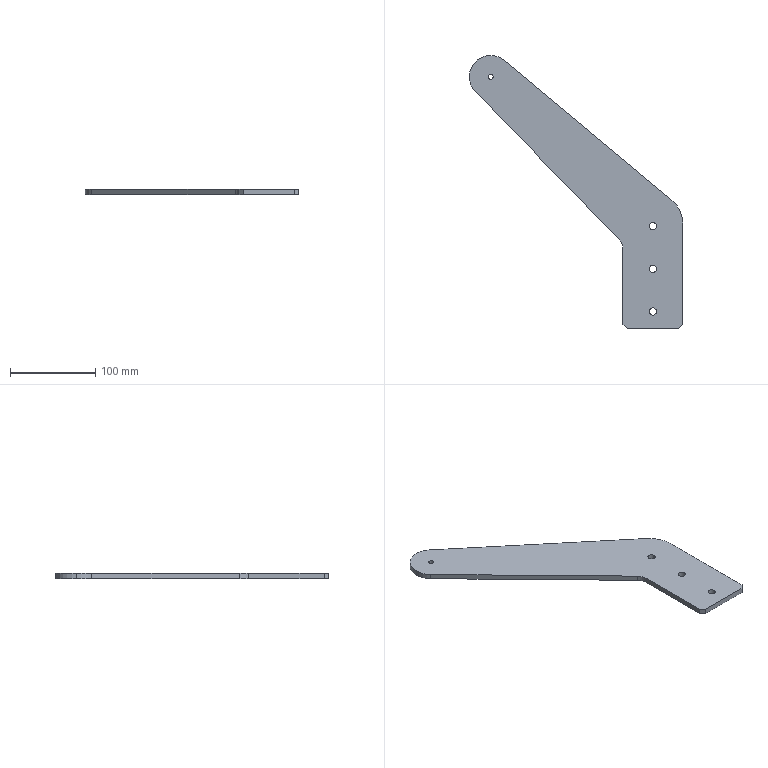Part | SolidWorks | features Chamfer 1, Extrusion 1 | 1 solid | 21 faces | box 250 x 320 x 6 mm | volume 153103 mm3 | cylinder 12 | plane 9 | commonest cylinder face diameters 8.5 x6 6 x2 50 x2 30 x1 70 x1
STEP:
#1=CARTESIAN_POINT('',(185.75,-175.,6.));
#2=VERTEX_POINT('',#1);
#3=CARTESIAN_POINT('',(194.25,-175.,6.));
#4=VERTEX_POINT('',#3);
#5=CARTESIAN_POINT('',(190.,-175.,6.));
#6=DIRECTION('',(0.,0.,1.));
#7=DIRECTION('',(1.,0.,0.));
#8=AXIS2_PLACEMENT_3D('',#5,#6,#7);
#9=CIRCLE('',#8,4.25);
#10=EDGE_CURVE('',#2,#4,#9,.T.);
#11=ORIENTED_EDGE('',*,*,#10,.T.);
#12=CARTESIAN_POINT('',(194.25,-175.,0.));
#13=VERTEX_POINT('',#12);
#14=CARTESIAN_POINT('',(194.25,-175.,6.));
#15=DIRECTION('',(0.,0.,-1.));
#16=VECTOR('',#15,1000.);
#17=LINE('',#14,#16);
#18=EDGE_CURVE('',#4,#13,#17,.T.);
#19=ORIENTED_EDGE('',*,*,#18,.T.);
#20=CARTESIAN_POINT('',(185.75,-175.,0.));
#21=VERTEX_POINT('',#20);
#22=CARTESIAN_POINT('',(190.,-175.,0.));
#23=DIRECTION('',(0.,0.,1.));
#24=DIRECTION('',(1.,0.,0.));
#25=AXIS2_PLACEMENT_3D('',#22,#23,#24);
#26=CIRCLE('',#25,4.25);
#27=EDGE_CURVE('',#21,#13,#26,.T.);
#28=ORIENTED_EDGE('',*,*,#27,.F.);
#29=CARTESIAN_POINT('',(185.75,-175.,6.));
#30=DIRECTION('',(0.,0.,-1.));
#31=VECTOR('',#30,1000.);
#32=LINE('',#29,#31);
#33=EDGE_CURVE('',#2,#21,#32,.T.);
#34=ORIENTED_EDGE('',*,*,#33,.F.);
#35=EDGE_LOOP('',(#11,#19,#28,#34));
#36=FACE_OUTER_BOUND('',#35,.T.);
#37=CARTESIAN_POINT('',(190.,-175.,6.));
#38=DIRECTION('',(0.,0.,-1.));
#39=DIRECTION('',(-1.,0.,0.));
#40=AXIS2_PLACEMENT_3D('',#37,#38,#39);
#41=CYLINDRICAL_SURFACE('',#40,4.25);
#42=ADVANCED_FACE('',(#36),#41,.F.);
#43=CARTESIAN_POINT('',(185.75,-225.,6.));
#44=VERTEX_POINT('',#43);
#45=CARTESIAN_POINT('',(194.25,-225.,6.));
#46=VERTEX_POINT('',#45);
#47=CARTESIAN_POINT('',(190.,-225.,6.));
#48=DIRECTION('',(0.,0.,1.));
#49=DIRECTION('',(1.,0.,0.));
#50=AXIS2_PLACEMENT_3D('',#47,#48,#49);
#51=CIRCLE('',#50,4.25);
#52=EDGE_CURVE('',#44,#46,#51,.T.);
#53=ORIENTED_EDGE('',*,*,#52,.T.);
#54=CARTESIAN_POINT('',(194.25,-225.,0.));
#55=VERTEX_POINT('',#54);
#56=CARTESIAN_POINT('',(194.25,-225.,6.));
#57=DIRECTION('',(0.,0.,-1.));
#58=VECTOR('',#57,1000.);
#59=LINE('',#56,#58);
#60=EDGE_CURVE('',#46,#55,#59,.T.);
#61=ORIENTED_EDGE('',*,*,#60,.T.);
#62=CARTESIAN_POINT('',(185.75,-225.,0.));
#63=VERTEX_POINT('',#62);
#64=CARTESIAN_POINT('',(190.,-225.,0.));
#65=DIRECTION('',(0.,0.,1.));
#66=DIRECTION('',(1.,0.,0.));
#67=AXIS2_PLACEMENT_3D('',#64,#65,#66);
#68=CIRCLE('',#67,4.25);
#69=EDGE_CURVE('',#63,#55,#68,.T.);
#70=ORIENTED_EDGE('',*,*,#69,.F.);
#71=CARTESIAN_POINT('',(185.75,-225.,6.));
#72=DIRECTION('',(0.,0.,-1.));
#73=VECTOR('',#72,1000.);
#74=LINE('',#71,#73);
#75=EDGE_CURVE('',#44,#63,#74,.T.);
#76=ORIENTED_EDGE('',*,*,#75,.F.);
#77=EDGE_LOOP('',(#53,#61,#70,#76));
#78=FACE_OUTER_BOUND('',#77,.T.);
#79=CARTESIAN_POINT('',(190.,-225.,6.));
#80=DIRECTION('',(0.,0.,-1.));
#81=DIRECTION('',(-1.,0.,0.));
#82=AXIS2_PLACEMENT_3D('',#79,#80,#81);
#83=CYLINDRICAL_SURFACE('',#82,4.25);
#84=ADVANCED_FACE('',(#78),#83,.F.);
#85=CARTESIAN_POINT('',(185.75,-275.,6.));
#86=VERTEX_POINT('',#85);
#87=CARTESIAN_POINT('',(194.25,-275.,6.));
#88=VERTEX_POINT('',#87);
#89=CARTESIAN_POINT('',(190.,-275.,6.));
#90=DIRECTION('',(0.,0.,1.));
#91=DIRECTION('',(1.,0.,0.));
#92=AXIS2_PLACEMENT_3D('',#89,#90,#91);
#93=CIRCLE('',#92,4.25);
#94=EDGE_CURVE('',#86,#88,#93,.T.);
#95=ORIENTED_EDGE('',*,*,#94,.T.);
#96=CARTESIAN_POINT('',(194.25,-275.,0.));
#97=VERTEX_POINT('',#96);
#98=CARTESIAN_POINT('',(194.25,-275.,6.));
#99=DIRECTION('',(0.,0.,-1.));
#100=VECTOR('',#99,1000.);
#101=LINE('',#98,#100);
#102=EDGE_CURVE('',#88,#97,#101,.T.);
#103=ORIENTED_EDGE('',*,*,#102,.T.);
#104=CARTESIAN_POINT('',(185.75,-275.,0.));
#105=VERTEX_POINT('',#104);
#106=CARTESIAN_POINT('',(190.,-275.,0.));
#107=DIRECTION('',(0.,0.,1.));
#108=DIRECTION('',(1.,0.,0.));
#109=AXIS2_PLACEMENT_3D('',#106,#107,#108);
#110=CIRCLE('',#109,4.25);
#111=EDGE_CURVE('',#105,#97,#110,.T.);
#112=ORIENTED_EDGE('',*,*,#111,.F.);
#113=CARTESIAN_POINT('',(185.75,-275.,6.));
#114=DIRECTION('',(0.,0.,-1.));
#115=VECTOR('',#114,1000.);
#116=LINE('',#113,#115);
#117=EDGE_CURVE('',#86,#105,#116,.T.);
#118=ORIENTED_EDGE('',*,*,#117,.F.);
#119=EDGE_LOOP('',(#95,#103,#112,#118));
#120=FACE_OUTER_BOUND('',#119,.T.);
#121=CARTESIAN_POINT('',(190.,-275.,6.));
#122=DIRECTION('',(0.,0.,-1.));
#123=DIRECTION('',(-1.,0.,0.));
#124=AXIS2_PLACEMENT_3D('',#121,#122,#123);
#125=CYLINDRICAL_SURFACE('',#124,4.25);
#126=ADVANCED_FACE('',(#120),#125,.F.);
#127=CARTESIAN_POINT('',(-3.,0.,6.));
#128=VERTEX_POINT('',#127);
#129=CARTESIAN_POINT('',(3.,0.,6.));
#130=VERTEX_POINT('',#129);
#131=CARTESIAN_POINT('',(0.,0.,6.));
#132=DIRECTION('',(0.,0.,1.));
#133=DIRECTION('',(1.,0.,0.));
#134=AXIS2_PLACEMENT_3D('',#131,#132,#133);
#135=CIRCLE('',#134,3.);
#136=EDGE_CURVE('',#128,#130,#135,.T.);
#137=ORIENTED_EDGE('',*,*,#136,.T.);
#138=CARTESIAN_POINT('',(3.,0.,0.));
#139=VERTEX_POINT('',#138);
#140=CARTESIAN_POINT('',(3.,0.,6.));
#141=DIRECTION('',(0.,0.,-1.));
#142=VECTOR('',#141,1000.);
#143=LINE('',#140,#142);
#144=EDGE_CURVE('',#130,#139,#143,.T.);
#145=ORIENTED_EDGE('',*,*,#144,.T.);
#146=CARTESIAN_POINT('',(-3.,0.,0.));
#147=VERTEX_POINT('',#146);
#148=CARTESIAN_POINT('',(0.,0.,0.));
#149=DIRECTION('',(0.,0.,1.));
#150=DIRECTION('',(1.,0.,0.));
#151=AXIS2_PLACEMENT_3D('',#148,#149,#150);
#152=CIRCLE('',#151,3.);
#153=EDGE_CURVE('',#147,#139,#152,.T.);
#154=ORIENTED_EDGE('',*,*,#153,.F.);
#155=CARTESIAN_POINT('',(-3.,0.,6.));
#156=DIRECTION('',(0.,0.,-1.));
#157=VECTOR('',#156,1000.);
#158=LINE('',#155,#157);
#159=EDGE_CURVE('',#128,#147,#158,.T.);
#160=ORIENTED_EDGE('',*,*,#159,.F.);
#161=EDGE_LOOP('',(#137,#145,#154,#160));
#162=FACE_OUTER_BOUND('',#161,.T.);
#163=CARTESIAN_POINT('',(0.,0.,6.));
#164=DIRECTION('',(0.,0.,-1.));
#165=DIRECTION('',(-1.,0.,0.));
#166=AXIS2_PLACEMENT_3D('',#163,#164,#165);
#167=CYLINDRICAL_SURFACE('',#166,3.);
#168=ADVANCED_FACE('',(#162),#167,.F.);
#169=CARTESIAN_POINT('',(-25.,0.,6.));
#170=VERTEX_POINT('',#169);
#171=CARTESIAN_POINT('',(-17.911,-17.442,6.));
#172=VERTEX_POINT('',#171);
#173=CARTESIAN_POINT('',(0.,0.,6.));
#174=DIRECTION('',(0.,0.,1.));
#175=DIRECTION('',(1.,0.,0.));
#176=AXIS2_PLACEMENT_3D('',#173,#174,#175);
#177=CIRCLE('',#176,25.);
#178=EDGE_CURVE('',#170,#172,#177,.T.);
#179=ORIENTED_EDGE('',*,*,#178,.F.);
#180=CARTESIAN_POINT('',(-25.,0.,0.));
#181=VERTEX_POINT('',#180);
#182=CARTESIAN_POINT('',(-25.,0.,6.));
#183=DIRECTION('',(0.,0.,-1.));
#184=VECTOR('',#183,1000.);
#185=LINE('',#182,#184);
#186=EDGE_CURVE('',#170,#181,#185,.T.);
#187=ORIENTED_EDGE('',*,*,#186,.T.);
#188=CARTESIAN_POINT('',(-17.911,-17.442,0.));
#189=VERTEX_POINT('',#188);
#190=CARTESIAN_POINT('',(0.,0.,0.));
#191=DIRECTION('',(0.,0.,1.));
#192=DIRECTION('',(1.,0.,0.));
#193=AXIS2_PLACEMENT_3D('',#190,#191,#192);
#194=CIRCLE('',#193,25.);
#195=EDGE_CURVE('',#181,#189,#194,.T.);
#196=ORIENTED_EDGE('',*,*,#195,.T.);
#197=CARTESIAN_POINT('',(-17.911,-17.442,6.));
#198=DIRECTION('',(0.,0.,-1.));
#199=VECTOR('',#198,1000.);
#200=LINE('',#197,#199);
#201=EDGE_CURVE('',#172,#189,#200,.T.);
#202=ORIENTED_EDGE('',*,*,#201,.F.);
#203=EDGE_LOOP('',(#179,#187,#196,#202));
#204=FACE_OUTER_BOUND('',#203,.T.);
#205=CARTESIAN_POINT('',(0.,0.,6.));
#206=DIRECTION('',(0.,0.,-1.));
#207=DIRECTION('',(-1.,0.,0.));
#208=AXIS2_PLACEMENT_3D('',#205,#206,#207);
#209=CYLINDRICAL_SURFACE('',#208,25.);
#210=ADVANCED_FACE('',(#204),#209,.T.);
#211=ORIENTED_EDGE('',*,*,#52,.F.);
#212=CARTESIAN_POINT('',(190.,-225.,6.));
#213=DIRECTION('',(0.,0.,1.));
#214=DIRECTION('',(1.,0.,0.));
#215=AXIS2_PLACEMENT_3D('',#212,#213,#214);
#216=CIRCLE('',#215,4.25);
#217=EDGE_CURVE('',#46,#44,#216,.T.);
#218=ORIENTED_EDGE('',*,*,#217,.F.);
#219=EDGE_LOOP('',(#211,#218));
#220=FACE_BOUND('',#219,.T.);
#221=ORIENTED_EDGE('',*,*,#136,.F.);
#222=CARTESIAN_POINT('',(0.,0.,6.));
#223=DIRECTION('',(0.,0.,1.));
#224=DIRECTION('',(1.,0.,0.));
#225=AXIS2_PLACEMENT_3D('',#222,#223,#224);
#226=CIRCLE('',#225,3.);
#227=EDGE_CURVE('',#130,#128,#226,.T.);
#228=ORIENTED_EDGE('',*,*,#227,.F.);
#229=EDGE_LOOP('',(#221,#228));
#230=FACE_BOUND('',#229,.T.);
#231=CARTESIAN_POINT('',(160.,-295.,6.));
#232=VERTEX_POINT('',#231);
#233=CARTESIAN_POINT('',(220.,-295.,6.));
#234=VERTEX_POINT('',#233);
#235=CARTESIAN_POINT('',(225.,-295.,6.));
#236=DIRECTION('',(1.,0.,0.));
#237=VECTOR('',#236,1000.);
#238=LINE('',#235,#237);
#239=EDGE_CURVE('',#232,#234,#238,.T.);
#240=ORIENTED_EDGE('',*,*,#239,.T.);
#241=CARTESIAN_POINT('',(225.,-290.,6.));
#242=VERTEX_POINT('',#241);
#243=CARTESIAN_POINT('',(257.5,-257.5,6.));
#244=DIRECTION('',(0.7071,0.7071,0.));
#245=VECTOR('',#244,1000.);
#246=LINE('',#243,#245);
#247=EDGE_CURVE('',#234,#242,#246,.T.);
#248=ORIENTED_EDGE('',*,*,#247,.T.);
#249=CARTESIAN_POINT('',(225.,-171.391,6.));
#250=VERTEX_POINT('',#249);
#251=CARTESIAN_POINT('',(225.,-171.391,6.));
#252=DIRECTION('',(0.,1.,0.));
#253=VECTOR('',#252,1000.);
#254=LINE('',#251,#253);
#255=EDGE_CURVE('',#242,#250,#254,.T.);
#256=ORIENTED_EDGE('',*,*,#255,.T.);
#257=CARTESIAN_POINT('',(212.41,-144.506,6.));
#258=VERTEX_POINT('',#257);
#259=CARTESIAN_POINT('',(190.,-171.391,6.));
#260=DIRECTION('',(0.,0.,1.));
#261=DIRECTION('',(-1.,0.,0.));
#262=AXIS2_PLACEMENT_3D('',#259,#260,#261);
#263=CIRCLE('',#262,35.);
#264=EDGE_CURVE('',#250,#258,#263,.T.);
#265=ORIENTED_EDGE('',*,*,#264,.T.);
#266=CARTESIAN_POINT('',(16.007,19.204,6.));
#267=VERTEX_POINT('',#266);
#268=CARTESIAN_POINT('',(16.007,19.204,6.));
#269=DIRECTION('',(-0.7681,0.6403,0.));
#270=VECTOR('',#269,1000.);
#271=LINE('',#268,#270);
#272=EDGE_CURVE('',#258,#267,#271,.T.);
#273=ORIENTED_EDGE('',*,*,#272,.T.);
#274=CARTESIAN_POINT('',(0.,0.,6.));
#275=DIRECTION('',(0.,0.,1.));
#276=DIRECTION('',(1.,0.,0.));
#277=AXIS2_PLACEMENT_3D('',#274,#275,#276);
#278=CIRCLE('',#277,25.);
#279=EDGE_CURVE('',#267,#170,#278,.T.);
#280=ORIENTED_EDGE('',*,*,#279,.T.);
#281=ORIENTED_EDGE('',*,*,#178,.T.);
#282=CARTESIAN_POINT('',(150.746,-190.632,6.));
#283=VERTEX_POINT('',#282);
#284=CARTESIAN_POINT('',(150.746,-190.632,6.));
#285=DIRECTION('',(0.6977,-0.7164,0.));
#286=VECTOR('',#285,1000.);
#287=LINE('',#284,#286);
#288=EDGE_CURVE('',#172,#283,#287,.T.);
#289=ORIENTED_EDGE('',*,*,#288,.T.);
#290=CARTESIAN_POINT('',(155.,-201.097,6.));
#291=VERTEX_POINT('',#290);
#292=CARTESIAN_POINT('',(140.,-201.097,6.));
#293=DIRECTION('',(0.,0.,-1.));
#294=DIRECTION('',(1.,0.,0.));
#295=AXIS2_PLACEMENT_3D('',#292,#293,#294);
#296=CIRCLE('',#295,15.);
#297=EDGE_CURVE('',#283,#291,#296,.T.);
#298=ORIENTED_EDGE('',*,*,#297,.T.);
#299=CARTESIAN_POINT('',(155.,-290.,6.));
#300=VERTEX_POINT('',#299);
#301=CARTESIAN_POINT('',(155.,-295.,6.));
#302=DIRECTION('',(0.,-1.,0.));
#303=VECTOR('',#302,1000.);
#304=LINE('',#301,#303);
#305=EDGE_CURVE('',#291,#300,#304,.T.);
#306=ORIENTED_EDGE('',*,*,#305,.T.);
#307=CARTESIAN_POINT('',(-67.5,-67.5,6.));
#308=DIRECTION('',(0.7071,-0.7071,0.));
#309=VECTOR('',#308,1000.);
#310=LINE('',#307,#309);
#311=EDGE_CURVE('',#300,#232,#310,.T.);
#312=ORIENTED_EDGE('',*,*,#311,.T.);
#313=EDGE_LOOP('',(#240,#248,#256,#265,#273,#280,#281,#289,#298,#306,#312));
#314=FACE_OUTER_BOUND('',#313,.T.);
#315=ORIENTED_EDGE('',*,*,#94,.F.);
#316=CARTESIAN_POINT('',(190.,-275.,6.));
#317=DIRECTION('',(0.,0.,1.));
#318=DIRECTION('',(1.,0.,0.));
#319=AXIS2_PLACEMENT_3D('',#316,#317,#318);
#320=CIRCLE('',#319,4.25);
#321=EDGE_CURVE('',#88,#86,#320,.T.);
#322=ORIENTED_EDGE('',*,*,#321,.F.);
#323=EDGE_LOOP('',(#315,#322));
#324=FACE_BOUND('',#323,.T.);
#325=ORIENTED_EDGE('',*,*,#10,.F.);
#326=CARTESIAN_POINT('',(190.,-175.,6.));
#327=DIRECTION('',(0.,0.,1.));
#328=DIRECTION('',(1.,0.,0.));
#329=AXIS2_PLACEMENT_3D('',#326,#327,#328);
#330=CIRCLE('',#329,4.25);
#331=EDGE_CURVE('',#4,#2,#330,.T.);
#332=ORIENTED_EDGE('',*,*,#331,.F.);
#333=EDGE_LOOP('',(#325,#332));
#334=FACE_BOUND('',#333,.T.);
#335=CARTESIAN_POINT('',(0.,0.,6.));
#336=DIRECTION('',(0.,0.,1.));
#337=DIRECTION('',(1.,0.,0.));
#338=AXIS2_PLACEMENT_3D('',#335,#336,#337);
#339=PLANE('',#338);
#340=ADVANCED_FACE('',(#220,#230,#314,#324,#334),#339,.T.);
#341=CARTESIAN_POINT('',(225.,-290.,0.));
#342=VERTEX_POINT('',#341);
#343=CARTESIAN_POINT('',(225.,-171.391,0.));
#344=VERTEX_POINT('',#343);
#345=CARTESIAN_POINT('',(225.,-171.391,0.));
#346=DIRECTION('',(0.,1.,0.));
#347=VECTOR('',#346,1000.);
#348=LINE('',#345,#347);
#349=EDGE_CURVE('',#342,#344,#348,.T.);
#350=ORIENTED_EDGE('',*,*,#349,.F.);
#351=CARTESIAN_POINT('',(220.,-295.,0.));
#352=VERTEX_POINT('',#351);
#353=CARTESIAN_POINT('',(225.,-290.,0.));
#354=DIRECTION('',(-0.7071,-0.7071,0.));
#355=VECTOR('',#354,1000.);
#356=LINE('',#353,#355);
#357=EDGE_CURVE('',#342,#352,#356,.T.);
#358=ORIENTED_EDGE('',*,*,#357,.T.);
#359=CARTESIAN_POINT('',(160.,-295.,0.));
#360=VERTEX_POINT('',#359);
#361=CARTESIAN_POINT('',(225.,-295.,0.));
#362=DIRECTION('',(1.,0.,0.));
#363=VECTOR('',#362,1000.);
#364=LINE('',#361,#363);
#365=EDGE_CURVE('',#360,#352,#364,.T.);
#366=ORIENTED_EDGE('',*,*,#365,.F.);
#367=CARTESIAN_POINT('',(155.,-290.,0.));
#368=VERTEX_POINT('',#367);
#369=CARTESIAN_POINT('',(160.,-295.,0.));
#370=DIRECTION('',(-0.7071,0.7071,0.));
#371=VECTOR('',#370,1000.);
#372=LINE('',#369,#371);
#373=EDGE_CURVE('',#360,#368,#372,.T.);
#374=ORIENTED_EDGE('',*,*,#373,.T.);
#375=CARTESIAN_POINT('',(155.,-201.097,0.));
#376=VERTEX_POINT('',#375);
#377=CARTESIAN_POINT('',(155.,-295.,0.));
#378=DIRECTION('',(0.,-1.,0.));
#379=VECTOR('',#378,1000.);
#380=LINE('',#377,#379);
#381=EDGE_CURVE('',#376,#368,#380,.T.);
#382=ORIENTED_EDGE('',*,*,#381,.F.);
#383=CARTESIAN_POINT('',(150.746,-190.632,0.));
#384=VERTEX_POINT('',#383);
#385=CARTESIAN_POINT('',(140.,-201.097,0.));
#386=DIRECTION('',(0.,0.,-1.));
#387=DIRECTION('',(1.,0.,0.));
#388=AXIS2_PLACEMENT_3D('',#385,#386,#387);
#389=CIRCLE('',#388,15.);
#390=EDGE_CURVE('',#384,#376,#389,.T.);
#391=ORIENTED_EDGE('',*,*,#390,.F.);
#392=CARTESIAN_POINT('',(150.746,-190.632,0.));
#393=DIRECTION('',(0.6977,-0.7164,0.));
#394=VECTOR('',#393,1000.);
#395=LINE('',#392,#394);
#396=EDGE_CURVE('',#189,#384,#395,.T.);
#397=ORIENTED_EDGE('',*,*,#396,.F.);
#398=ORIENTED_EDGE('',*,*,#195,.F.);
#399=CARTESIAN_POINT('',(16.007,19.204,0.));
#400=VERTEX_POINT('',#399);
#401=CARTESIAN_POINT('',(0.,0.,0.));
#402=DIRECTION('',(0.,0.,1.));
#403=DIRECTION('',(1.,0.,0.));
#404=AXIS2_PLACEMENT_3D('',#401,#402,#403);
#405=CIRCLE('',#404,25.);
#406=EDGE_CURVE('',#400,#181,#405,.T.);
#407=ORIENTED_EDGE('',*,*,#406,.F.);
#408=CARTESIAN_POINT('',(212.41,-144.506,0.));
#409=VERTEX_POINT('',#408);
#410=CARTESIAN_POINT('',(16.007,19.204,0.));
#411=DIRECTION('',(-0.7681,0.6403,0.));
#412=VECTOR('',#411,1000.);
#413=LINE('',#410,#412);
#414=EDGE_CURVE('',#409,#400,#413,.T.);
#415=ORIENTED_EDGE('',*,*,#414,.F.);
#416=CARTESIAN_POINT('',(190.,-171.391,0.));
#417=DIRECTION('',(0.,0.,1.));
#418=DIRECTION('',(-1.,0.,0.));
#419=AXIS2_PLACEMENT_3D('',#416,#417,#418);
#420=CIRCLE('',#419,35.);
#421=EDGE_CURVE('',#344,#409,#420,.T.);
#422=ORIENTED_EDGE('',*,*,#421,.F.);
#423=EDGE_LOOP('',(#350,#358,#366,#374,#382,#391,#397,#398,#407,#415,#422));
#424=FACE_OUTER_BOUND('',#423,.T.);
#425=ORIENTED_EDGE('',*,*,#153,.T.);
#426=CARTESIAN_POINT('',(0.,0.,0.));
#427=DIRECTION('',(0.,0.,1.));
#428=DIRECTION('',(1.,0.,0.));
#429=AXIS2_PLACEMENT_3D('',#426,#427,#428);
#430=CIRCLE('',#429,3.);
#431=EDGE_CURVE('',#139,#147,#430,.T.);
#432=ORIENTED_EDGE('',*,*,#431,.T.);
#433=EDGE_LOOP('',(#425,#432));
#434=FACE_BOUND('',#433,.T.);
#435=ORIENTED_EDGE('',*,*,#111,.T.);
#436=CARTESIAN_POINT('',(190.,-275.,0.));
#437=DIRECTION('',(0.,0.,1.));
#438=DIRECTION('',(1.,0.,0.));
#439=AXIS2_PLACEMENT_3D('',#436,#437,#438);
#440=CIRCLE('',#439,4.25);
#441=EDGE_CURVE('',#97,#105,#440,.T.);
#442=ORIENTED_EDGE('',*,*,#441,.T.);
#443=EDGE_LOOP('',(#435,#442));
#444=FACE_BOUND('',#443,.T.);
#445=ORIENTED_EDGE('',*,*,#69,.T.);
#446=CARTESIAN_POINT('',(190.,-225.,0.));
#447=DIRECTION('',(0.,0.,1.));
#448=DIRECTION('',(1.,0.,0.));
#449=AXIS2_PLACEMENT_3D('',#446,#447,#448);
#450=CIRCLE('',#449,4.25);
#451=EDGE_CURVE('',#55,#63,#450,.T.);
#452=ORIENTED_EDGE('',*,*,#451,.T.);
#453=EDGE_LOOP('',(#445,#452));
#454=FACE_BOUND('',#453,.T.);
#455=ORIENTED_EDGE('',*,*,#27,.T.);
#456=CARTESIAN_POINT('',(190.,-175.,0.));
#457=DIRECTION('',(0.,0.,1.));
#458=DIRECTION('',(1.,0.,0.));
#459=AXIS2_PLACEMENT_3D('',#456,#457,#458);
#460=CIRCLE('',#459,4.25);
#461=EDGE_CURVE('',#13,#21,#460,.T.);
#462=ORIENTED_EDGE('',*,*,#461,.T.);
#463=EDGE_LOOP('',(#455,#462));
#464=FACE_BOUND('',#463,.T.);
#465=CARTESIAN_POINT('',(0.,0.,0.));
#466=DIRECTION('',(0.,0.,1.));
#467=DIRECTION('',(1.,0.,0.));
#468=AXIS2_PLACEMENT_3D('',#465,#466,#467);
#469=PLANE('',#468);
#470=ADVANCED_FACE('',(#424,#434,#444,#454,#464),#469,.F.);
#471=ORIENTED_EDGE('',*,*,#186,.F.);
#472=ORIENTED_EDGE('',*,*,#279,.F.);
#473=CARTESIAN_POINT('',(16.007,19.204,6.));
#474=DIRECTION('',(0.,0.,-1.));
#475=VECTOR('',#474,1000.);
#476=LINE('',#473,#475);
#477=EDGE_CURVE('',#267,#400,#476,.T.);
#478=ORIENTED_EDGE('',*,*,#477,.T.);
#479=ORIENTED_EDGE('',*,*,#406,.T.);
#480=EDGE_LOOP('',(#471,#472,#478,#479));
#481=FACE_OUTER_BOUND('',#480,.T.);
#482=CARTESIAN_POINT('',(0.,0.,6.));
#483=DIRECTION('',(0.,0.,-1.));
#484=DIRECTION('',(-1.,0.,0.));
#485=AXIS2_PLACEMENT_3D('',#482,#483,#484);
#486=CYLINDRICAL_SURFACE('',#485,25.);
#487=ADVANCED_FACE('',(#481),#486,.T.);
#488=ORIENTED_EDGE('',*,*,#396,.T.);
#489=CARTESIAN_POINT('',(150.746,-190.632,6.));
#490=DIRECTION('',(0.,0.,-1.));
#491=VECTOR('',#490,1000.);
#492=LINE('',#489,#491);
#493=EDGE_CURVE('',#283,#384,#492,.T.);
#494=ORIENTED_EDGE('',*,*,#493,.F.);
#495=ORIENTED_EDGE('',*,*,#288,.F.);
#496=ORIENTED_EDGE('',*,*,#201,.T.);
#497=EDGE_LOOP('',(#488,#494,#495,#496));
#498=FACE_OUTER_BOUND('',#497,.T.);
#499=CARTESIAN_POINT('',(150.746,-190.632,6.));
#500=DIRECTION('',(0.7164,0.6977,0.));
#501=DIRECTION('',(-0.6977,0.7164,0.));
#502=AXIS2_PLACEMENT_3D('',#499,#500,#501);
#503=PLANE('',#502);
#504=ADVANCED_FACE('',(#498),#503,.F.);
#505=ORIENTED_EDGE('',*,*,#390,.T.);
#506=CARTESIAN_POINT('',(155.,-201.097,6.));
#507=DIRECTION('',(0.,0.,-1.));
#508=VECTOR('',#507,1000.);
#509=LINE('',#506,#508);
#510=EDGE_CURVE('',#291,#376,#509,.T.);
#511=ORIENTED_EDGE('',*,*,#510,.F.);
#512=ORIENTED_EDGE('',*,*,#297,.F.);
#513=ORIENTED_EDGE('',*,*,#493,.T.);
#514=EDGE_LOOP('',(#505,#511,#512,#513));
#515=FACE_OUTER_BOUND('',#514,.T.);
#516=CARTESIAN_POINT('',(140.,-201.097,6.));
#517=DIRECTION('',(0.,0.,-1.));
#518=DIRECTION('',(-1.,0.,0.));
#519=AXIS2_PLACEMENT_3D('',#516,#517,#518);
#520=CYLINDRICAL_SURFACE('',#519,15.);
#521=ADVANCED_FACE('',(#515),#520,.F.);
#522=ORIENTED_EDGE('',*,*,#381,.T.);
#523=CARTESIAN_POINT('',(155.,-290.,6.));
#524=DIRECTION('',(0.,0.,1.));
#525=VECTOR('',#524,1000.);
#526=LINE('',#523,#525);
#527=EDGE_CURVE('',#368,#300,#526,.T.);
#528=ORIENTED_EDGE('',*,*,#527,.T.);
#529=ORIENTED_EDGE('',*,*,#305,.F.);
#530=ORIENTED_EDGE('',*,*,#510,.T.);
#531=EDGE_LOOP('',(#522,#528,#529,#530));
#532=FACE_OUTER_BOUND('',#531,.T.);
#533=CARTESIAN_POINT('',(155.,-295.,6.));
#534=DIRECTION('',(1.,0.,0.));
#535=DIRECTION('',(0.,0.,-1.));
#536=AXIS2_PLACEMENT_3D('',#533,#534,#535);
#537=PLANE('',#536);
#538=ADVANCED_FACE('',(#532),#537,.F.);
#539=ORIENTED_EDGE('',*,*,#365,.T.);
#540=CARTESIAN_POINT('',(220.,-295.,6.));
#541=DIRECTION('',(0.,0.,1.));
#542=VECTOR('',#541,1000.);
#543=LINE('',#540,#542);
#544=EDGE_CURVE('',#352,#234,#543,.T.);
#545=ORIENTED_EDGE('',*,*,#544,.T.);
#546=ORIENTED_EDGE('',*,*,#239,.F.);
#547=CARTESIAN_POINT('',(160.,-295.,6.));
#548=DIRECTION('',(0.,0.,-1.));
#549=VECTOR('',#548,1000.);
#550=LINE('',#547,#549);
#551=EDGE_CURVE('',#232,#360,#550,.T.);
#552=ORIENTED_EDGE('',*,*,#551,.T.);
#553=EDGE_LOOP('',(#539,#545,#546,#552));
#554=FACE_OUTER_BOUND('',#553,.T.);
#555=CARTESIAN_POINT('',(225.,-295.,6.));
#556=DIRECTION('',(0.,1.,0.));
#557=DIRECTION('',(0.,0.,1.));
#558=AXIS2_PLACEMENT_3D('',#555,#556,#557);
#559=PLANE('',#558);
#560=ADVANCED_FACE('',(#554),#559,.F.);
#561=ORIENTED_EDGE('',*,*,#255,.F.);
#562=CARTESIAN_POINT('',(225.,-290.,6.));
#563=DIRECTION('',(0.,0.,-1.));
#564=VECTOR('',#563,1000.);
#565=LINE('',#562,#564);
#566=EDGE_CURVE('',#242,#342,#565,.T.);
#567=ORIENTED_EDGE('',*,*,#566,.T.);
#568=ORIENTED_EDGE('',*,*,#349,.T.);
#569=CARTESIAN_POINT('',(225.,-171.391,6.));
#570=DIRECTION('',(0.,0.,-1.));
#571=VECTOR('',#570,1000.);
#572=LINE('',#569,#571);
#573=EDGE_CURVE('',#250,#344,#572,.T.);
#574=ORIENTED_EDGE('',*,*,#573,.F.);
#575=EDGE_LOOP('',(#561,#567,#568,#574));
#576=FACE_OUTER_BOUND('',#575,.T.);
#577=CARTESIAN_POINT('',(225.,-171.391,6.));
#578=DIRECTION('',(-1.,0.,0.));
#579=DIRECTION('',(0.,0.,1.));
#580=AXIS2_PLACEMENT_3D('',#577,#578,#579);
#581=PLANE('',#580);
#582=ADVANCED_FACE('',(#576),#581,.F.);
#583=ORIENTED_EDGE('',*,*,#421,.T.);
#584=CARTESIAN_POINT('',(212.41,-144.506,6.));
#585=DIRECTION('',(0.,0.,-1.));
#586=VECTOR('',#585,1000.);
#587=LINE('',#584,#586);
#588=EDGE_CURVE('',#258,#409,#587,.T.);
#589=ORIENTED_EDGE('',*,*,#588,.F.);
#590=ORIENTED_EDGE('',*,*,#264,.F.);
#591=ORIENTED_EDGE('',*,*,#573,.T.);
#592=EDGE_LOOP('',(#583,#589,#590,#591));
#593=FACE_OUTER_BOUND('',#592,.T.);
#594=CARTESIAN_POINT('',(190.,-171.391,6.));
#595=DIRECTION('',(0.,0.,-1.));
#596=DIRECTION('',(-1.,0.,0.));
#597=AXIS2_PLACEMENT_3D('',#594,#595,#596);
#598=CYLINDRICAL_SURFACE('',#597,35.);
#599=ADVANCED_FACE('',(#593),#598,.T.);
#600=ORIENTED_EDGE('',*,*,#414,.T.);
#601=ORIENTED_EDGE('',*,*,#477,.F.);
#602=ORIENTED_EDGE('',*,*,#272,.F.);
#603=ORIENTED_EDGE('',*,*,#588,.T.);
#604=EDGE_LOOP('',(#600,#601,#602,#603));
#605=FACE_OUTER_BOUND('',#604,.T.);
#606=CARTESIAN_POINT('',(16.007,19.204,6.));
#607=DIRECTION('',(-0.6403,-0.7681,0.));
#608=DIRECTION('',(0.7681,-0.6403,0.));
#609=AXIS2_PLACEMENT_3D('',#606,#607,#608);
#610=PLANE('',#609);
#611=ADVANCED_FACE('',(#605),#610,.F.);
#612=ORIENTED_EDGE('',*,*,#144,.F.);
#613=ORIENTED_EDGE('',*,*,#227,.T.);
#614=ORIENTED_EDGE('',*,*,#159,.T.);
#615=ORIENTED_EDGE('',*,*,#431,.F.);
#616=EDGE_LOOP('',(#612,#613,#614,#615));
#617=FACE_OUTER_BOUND('',#616,.T.);
#618=CARTESIAN_POINT('',(0.,0.,6.));
#619=DIRECTION('',(0.,0.,-1.));
#620=DIRECTION('',(-1.,0.,0.));
#621=AXIS2_PLACEMENT_3D('',#618,#619,#620);
#622=CYLINDRICAL_SURFACE('',#621,3.);
#623=ADVANCED_FACE('',(#617),#622,.F.);
#624=ORIENTED_EDGE('',*,*,#102,.F.);
#625=ORIENTED_EDGE('',*,*,#321,.T.);
#626=ORIENTED_EDGE('',*,*,#117,.T.);
#627=ORIENTED_EDGE('',*,*,#441,.F.);
#628=EDGE_LOOP('',(#624,#625,#626,#627));
#629=FACE_OUTER_BOUND('',#628,.T.);
#630=CARTESIAN_POINT('',(190.,-275.,6.));
#631=DIRECTION('',(0.,0.,-1.));
#632=DIRECTION('',(-1.,0.,0.));
#633=AXIS2_PLACEMENT_3D('',#630,#631,#632);
#634=CYLINDRICAL_SURFACE('',#633,4.25);
#635=ADVANCED_FACE('',(#629),#634,.F.);
#636=ORIENTED_EDGE('',*,*,#60,.F.);
#637=ORIENTED_EDGE('',*,*,#217,.T.);
#638=ORIENTED_EDGE('',*,*,#75,.T.);
#639=ORIENTED_EDGE('',*,*,#451,.F.);
#640=EDGE_LOOP('',(#636,#637,#638,#639));
#641=FACE_OUTER_BOUND('',#640,.T.);
#642=CARTESIAN_POINT('',(190.,-225.,6.));
#643=DIRECTION('',(0.,0.,-1.));
#644=DIRECTION('',(-1.,0.,0.));
#645=AXIS2_PLACEMENT_3D('',#642,#643,#644);
#646=CYLINDRICAL_SURFACE('',#645,4.25);
#647=ADVANCED_FACE('',(#641),#646,.F.);
#648=ORIENTED_EDGE('',*,*,#18,.F.);
#649=ORIENTED_EDGE('',*,*,#331,.T.);
#650=ORIENTED_EDGE('',*,*,#33,.T.);
#651=ORIENTED_EDGE('',*,*,#461,.F.);
#652=EDGE_LOOP('',(#648,#649,#650,#651));
#653=FACE_OUTER_BOUND('',#652,.T.);
#654=CARTESIAN_POINT('',(190.,-175.,6.));
#655=DIRECTION('',(0.,0.,-1.));
#656=DIRECTION('',(-1.,0.,0.));
#657=AXIS2_PLACEMENT_3D('',#654,#655,#656);
#658=CYLINDRICAL_SURFACE('',#657,4.25);
#659=ADVANCED_FACE('',(#653),#658,.F.);
#660=ORIENTED_EDGE('',*,*,#247,.F.);
#661=ORIENTED_EDGE('',*,*,#544,.F.);
#662=ORIENTED_EDGE('',*,*,#357,.F.);
#663=ORIENTED_EDGE('',*,*,#566,.F.);
#664=EDGE_LOOP('',(#660,#661,#662,#663));
#665=FACE_OUTER_BOUND('',#664,.T.);
#666=CARTESIAN_POINT('',(225.,-290.,6.));
#667=DIRECTION('',(-0.7071,0.7071,0.));
#668=DIRECTION('',(0.,0.,-1.));
#669=AXIS2_PLACEMENT_3D('',#666,#667,#668);
#670=PLANE('',#669);
#671=ADVANCED_FACE('',(#665),#670,.F.);
#672=ORIENTED_EDGE('',*,*,#311,.F.);
#673=ORIENTED_EDGE('',*,*,#527,.F.);
#674=ORIENTED_EDGE('',*,*,#373,.F.);
#675=ORIENTED_EDGE('',*,*,#551,.F.);
#676=EDGE_LOOP('',(#672,#673,#674,#675));
#677=FACE_OUTER_BOUND('',#676,.T.);
#678=CARTESIAN_POINT('',(160.,-295.,6.));
#679=DIRECTION('',(0.7071,0.7071,0.));
#680=DIRECTION('',(0.,0.,-1.));
#681=AXIS2_PLACEMENT_3D('',#678,#679,#680);
#682=PLANE('',#681);
#683=ADVANCED_FACE('',(#677),#682,.F.);
#684=CLOSED_SHELL('',(#42,#84,#126,#168,#210,#340,#470,#487,#504,#521,#538,#560,#582,#599,#611,#623,#635,#647,#659,#671,#683));
#685=MANIFOLD_SOLID_BREP('',#684);
#686=CARTESIAN_POINT('',(0.,0.,0.));
#687=DIRECTION('',(0.,0.,1.));
#688=DIRECTION('',(1.,0.,0.));
#689=AXIS2_PLACEMENT_3D('',#686,#687,#688);
#690=(LENGTH_UNIT()NAMED_UNIT(*)SI_UNIT(.MILLI.,.METRE.));
#691=UNCERTAINTY_MEASURE_WITH_UNIT(LENGTH_MEASURE(0.00001),#690,'','');
#692=(NAMED_UNIT(*)PLANE_ANGLE_UNIT()SI_UNIT($,.RADIAN.));
#693=(NAMED_UNIT(*)SI_UNIT($,.STERADIAN.)SOLID_ANGLE_UNIT());
#694=(GEOMETRIC_REPRESENTATION_CONTEXT(3)GLOBAL_UNCERTAINTY_ASSIGNED_CONTEXT((#691))GLOBAL_UNIT_ASSIGNED_CONTEXT((#690,#692,#693))REPRESENTATION_CONTEXT('',''));
#695=ADVANCED_BREP_SHAPE_REPRESENTATION('',(#685,#689),#694);